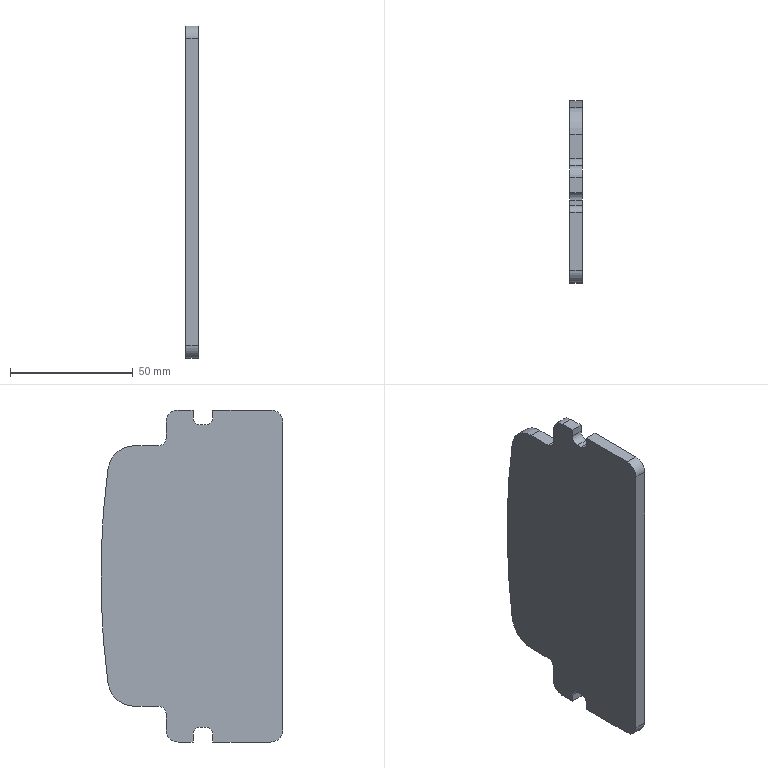Part | SolidWorks | features BaseBody 1 | 1 solid | 30 faces | box 5 x 74 x 135 mm | volume 44638 mm3 | plane 17 | cylinder 13 | commonest cylinder face diameters 6 x6 10 x4 22 x2 660 x1
STEP:
#1=CARTESIAN_POINT('',(616.,51.,53.));
#2=VERTEX_POINT('',#1);
#3=CARTESIAN_POINT('',(616.,48.,56.));
#4=VERTEX_POINT('',#3);
#5=CARTESIAN_POINT('',(616.,51.,56.));
#6=DIRECTION('',(-1.,0.,0.));
#7=DIRECTION('',(0.,0.,-1.));
#8=AXIS2_PLACEMENT_3D('',#5,#6,#7);
#9=CIRCLE('',#8,3.);
#10=EDGE_CURVE('',#2,#4,#9,.T.);
#11=ORIENTED_EDGE('',*,*,#10,.T.);
#12=CARTESIAN_POINT('',(616.,48.,62.5));
#13=VERTEX_POINT('',#12);
#14=CARTESIAN_POINT('',(616.,48.,62.5));
#15=DIRECTION('',(0.,0.,1.));
#16=VECTOR('',#15,1000.);
#17=LINE('',#14,#16);
#18=EDGE_CURVE('',#4,#13,#17,.T.);
#19=ORIENTED_EDGE('',*,*,#18,.T.);
#20=CARTESIAN_POINT('',(616.,43.,67.5));
#21=VERTEX_POINT('',#20);
#22=CARTESIAN_POINT('',(616.,43.,62.5));
#23=DIRECTION('',(1.,0.,0.));
#24=DIRECTION('',(0.,0.,-1.));
#25=AXIS2_PLACEMENT_3D('',#22,#23,#24);
#26=CIRCLE('',#25,5.);
#27=EDGE_CURVE('',#13,#21,#26,.T.);
#28=ORIENTED_EDGE('',*,*,#27,.T.);
#29=CARTESIAN_POINT('',(616.,37.,67.5));
#30=VERTEX_POINT('',#29);
#31=CARTESIAN_POINT('',(616.,43.,67.5));
#32=DIRECTION('',(0.,-1.,0.));
#33=VECTOR('',#32,1000.);
#34=LINE('',#31,#33);
#35=EDGE_CURVE('',#21,#30,#34,.T.);
#36=ORIENTED_EDGE('',*,*,#35,.T.);
#37=CARTESIAN_POINT('',(616.,37.,64.5));
#38=VERTEX_POINT('',#37);
#39=CARTESIAN_POINT('',(616.,37.,62.5));
#40=DIRECTION('',(0.,0.,-1.));
#41=VECTOR('',#40,1000.);
#42=LINE('',#39,#41);
#43=EDGE_CURVE('',#30,#38,#42,.T.);
#44=ORIENTED_EDGE('',*,*,#43,.T.);
#45=CARTESIAN_POINT('',(616.,34.,61.5));
#46=VERTEX_POINT('',#45);
#47=CARTESIAN_POINT('',(616.,34.,64.5));
#48=DIRECTION('',(-1.,0.,0.));
#49=DIRECTION('',(0.,0.,-1.));
#50=AXIS2_PLACEMENT_3D('',#47,#48,#49);
#51=CIRCLE('',#50,3.);
#52=EDGE_CURVE('',#38,#46,#51,.T.);
#53=ORIENTED_EDGE('',*,*,#52,.T.);
#54=CARTESIAN_POINT('',(616.,32.,61.5));
#55=VERTEX_POINT('',#54);
#56=CARTESIAN_POINT('',(616.,43.,61.5));
#57=DIRECTION('',(0.,-1.,0.));
#58=VECTOR('',#57,1000.);
#59=LINE('',#56,#58);
#60=EDGE_CURVE('',#46,#55,#59,.T.);
#61=ORIENTED_EDGE('',*,*,#60,.T.);
#62=CARTESIAN_POINT('',(616.,29.,64.5));
#63=VERTEX_POINT('',#62);
#64=CARTESIAN_POINT('',(616.,32.,64.5));
#65=DIRECTION('',(-1.,0.,0.));
#66=DIRECTION('',(0.,0.,-1.));
#67=AXIS2_PLACEMENT_3D('',#64,#65,#66);
#68=CIRCLE('',#67,3.);
#69=EDGE_CURVE('',#55,#63,#68,.T.);
#70=ORIENTED_EDGE('',*,*,#69,.T.);
#71=CARTESIAN_POINT('',(616.,29.,67.5));
#72=VERTEX_POINT('',#71);
#73=CARTESIAN_POINT('',(616.,29.,62.5));
#74=DIRECTION('',(0.,0.,1.));
#75=VECTOR('',#74,1000.);
#76=LINE('',#73,#75);
#77=EDGE_CURVE('',#63,#72,#76,.T.);
#78=ORIENTED_EDGE('',*,*,#77,.T.);
#79=CARTESIAN_POINT('',(616.,5.5,67.5));
#80=VERTEX_POINT('',#79);
#81=CARTESIAN_POINT('',(616.,43.,67.5));
#82=DIRECTION('',(0.,-1.,0.));
#83=VECTOR('',#82,1000.);
#84=LINE('',#81,#83);
#85=EDGE_CURVE('',#72,#80,#84,.T.);
#86=ORIENTED_EDGE('',*,*,#85,.T.);
#87=CARTESIAN_POINT('',(616.,0.5,62.5));
#88=VERTEX_POINT('',#87);
#89=CARTESIAN_POINT('',(616.,5.5,62.5));
#90=DIRECTION('',(1.,0.,0.));
#91=DIRECTION('',(0.,0.,-1.));
#92=AXIS2_PLACEMENT_3D('',#89,#90,#91);
#93=CIRCLE('',#92,5.);
#94=EDGE_CURVE('',#80,#88,#93,.T.);
#95=ORIENTED_EDGE('',*,*,#94,.T.);
#96=CARTESIAN_POINT('',(616.,0.5,-62.5));
#97=VERTEX_POINT('',#96);
#98=CARTESIAN_POINT('',(616.,0.5,62.5));
#99=DIRECTION('',(0.,0.,-1.));
#100=VECTOR('',#99,1000.);
#101=LINE('',#98,#100);
#102=EDGE_CURVE('',#88,#97,#101,.T.);
#103=ORIENTED_EDGE('',*,*,#102,.T.);
#104=CARTESIAN_POINT('',(616.,5.5,-67.5));
#105=VERTEX_POINT('',#104);
#106=CARTESIAN_POINT('',(616.,5.5,-62.5));
#107=DIRECTION('',(1.,0.,0.));
#108=DIRECTION('',(0.,0.,-1.));
#109=AXIS2_PLACEMENT_3D('',#106,#107,#108);
#110=CIRCLE('',#109,5.);
#111=EDGE_CURVE('',#97,#105,#110,.T.);
#112=ORIENTED_EDGE('',*,*,#111,.T.);
#113=CARTESIAN_POINT('',(616.,29.,-67.5));
#114=VERTEX_POINT('',#113);
#115=CARTESIAN_POINT('',(616.,43.,-67.5));
#116=DIRECTION('',(0.,1.,0.));
#117=VECTOR('',#116,1000.);
#118=LINE('',#115,#117);
#119=EDGE_CURVE('',#105,#114,#118,.T.);
#120=ORIENTED_EDGE('',*,*,#119,.T.);
#121=CARTESIAN_POINT('',(616.,29.,-64.5));
#122=VERTEX_POINT('',#121);
#123=CARTESIAN_POINT('',(616.,29.,62.5));
#124=DIRECTION('',(0.,0.,1.));
#125=VECTOR('',#124,1000.);
#126=LINE('',#123,#125);
#127=EDGE_CURVE('',#114,#122,#126,.T.);
#128=ORIENTED_EDGE('',*,*,#127,.T.);
#129=CARTESIAN_POINT('',(616.,32.,-61.5));
#130=VERTEX_POINT('',#129);
#131=CARTESIAN_POINT('',(616.,32.,-64.5));
#132=DIRECTION('',(-1.,0.,0.));
#133=DIRECTION('',(0.,0.,-1.));
#134=AXIS2_PLACEMENT_3D('',#131,#132,#133);
#135=CIRCLE('',#134,3.);
#136=EDGE_CURVE('',#122,#130,#135,.T.);
#137=ORIENTED_EDGE('',*,*,#136,.T.);
#138=CARTESIAN_POINT('',(616.,34.,-61.5));
#139=VERTEX_POINT('',#138);
#140=CARTESIAN_POINT('',(616.,43.,-61.5));
#141=DIRECTION('',(0.,1.,0.));
#142=VECTOR('',#141,1000.);
#143=LINE('',#140,#142);
#144=EDGE_CURVE('',#130,#139,#143,.T.);
#145=ORIENTED_EDGE('',*,*,#144,.T.);
#146=CARTESIAN_POINT('',(616.,37.,-64.5));
#147=VERTEX_POINT('',#146);
#148=CARTESIAN_POINT('',(616.,34.,-64.5));
#149=DIRECTION('',(-1.,0.,0.));
#150=DIRECTION('',(0.,0.,-1.));
#151=AXIS2_PLACEMENT_3D('',#148,#149,#150);
#152=CIRCLE('',#151,3.);
#153=EDGE_CURVE('',#139,#147,#152,.T.);
#154=ORIENTED_EDGE('',*,*,#153,.T.);
#155=CARTESIAN_POINT('',(616.,37.,-67.5));
#156=VERTEX_POINT('',#155);
#157=CARTESIAN_POINT('',(616.,37.,62.5));
#158=DIRECTION('',(0.,0.,-1.));
#159=VECTOR('',#158,1000.);
#160=LINE('',#157,#159);
#161=EDGE_CURVE('',#147,#156,#160,.T.);
#162=ORIENTED_EDGE('',*,*,#161,.T.);
#163=CARTESIAN_POINT('',(616.,43.,-67.5));
#164=VERTEX_POINT('',#163);
#165=CARTESIAN_POINT('',(616.,43.,-67.5));
#166=DIRECTION('',(0.,1.,0.));
#167=VECTOR('',#166,1000.);
#168=LINE('',#165,#167);
#169=EDGE_CURVE('',#156,#164,#168,.T.);
#170=ORIENTED_EDGE('',*,*,#169,.T.);
#171=CARTESIAN_POINT('',(616.,48.,-62.5));
#172=VERTEX_POINT('',#171);
#173=CARTESIAN_POINT('',(616.,43.,-62.5));
#174=DIRECTION('',(1.,0.,0.));
#175=DIRECTION('',(0.,0.,-1.));
#176=AXIS2_PLACEMENT_3D('',#173,#174,#175);
#177=CIRCLE('',#176,5.);
#178=EDGE_CURVE('',#164,#172,#177,.T.);
#179=ORIENTED_EDGE('',*,*,#178,.T.);
#180=CARTESIAN_POINT('',(616.,48.,-56.));
#181=VERTEX_POINT('',#180);
#182=CARTESIAN_POINT('',(616.,48.,62.5));
#183=DIRECTION('',(0.,0.,1.));
#184=VECTOR('',#183,1000.);
#185=LINE('',#182,#184);
#186=EDGE_CURVE('',#172,#181,#185,.T.);
#187=ORIENTED_EDGE('',*,*,#186,.T.);
#188=CARTESIAN_POINT('',(616.,51.,-53.));
#189=VERTEX_POINT('',#188);
#190=CARTESIAN_POINT('',(616.,51.,-56.));
#191=DIRECTION('',(-1.,0.,0.));
#192=DIRECTION('',(0.,0.,-1.));
#193=AXIS2_PLACEMENT_3D('',#190,#191,#192);
#194=CIRCLE('',#193,3.);
#195=EDGE_CURVE('',#181,#189,#194,.T.);
#196=ORIENTED_EDGE('',*,*,#195,.T.);
#197=CARTESIAN_POINT('',(616.,60.723,-53.));
#198=VERTEX_POINT('',#197);
#199=CARTESIAN_POINT('',(616.,43.,-53.));
#200=DIRECTION('',(0.,1.,0.));
#201=VECTOR('',#200,1000.);
#202=LINE('',#199,#201);
#203=EDGE_CURVE('',#189,#198,#202,.T.);
#204=ORIENTED_EDGE('',*,*,#203,.T.);
#205=CARTESIAN_POINT('',(616.,71.627,-43.448));
#206=VERTEX_POINT('',#205);
#207=CARTESIAN_POINT('',(616.,60.723,-42.));
#208=DIRECTION('',(1.,0.,0.));
#209=DIRECTION('',(0.,0.,-1.));
#210=AXIS2_PLACEMENT_3D('',#207,#208,#209);
#211=CIRCLE('',#210,11.);
#212=EDGE_CURVE('',#198,#206,#211,.T.);
#213=ORIENTED_EDGE('',*,*,#212,.T.);
#214=CARTESIAN_POINT('',(616.,71.627,43.448));
#215=VERTEX_POINT('',#214);
#216=CARTESIAN_POINT('',(616.,-255.5,0.));
#217=DIRECTION('',(1.,0.,0.));
#218=DIRECTION('',(0.,0.,-1.));
#219=AXIS2_PLACEMENT_3D('',#216,#217,#218);
#220=CIRCLE('',#219,330.);
#221=EDGE_CURVE('',#206,#215,#220,.T.);
#222=ORIENTED_EDGE('',*,*,#221,.T.);
#223=CARTESIAN_POINT('',(616.,60.723,53.));
#224=VERTEX_POINT('',#223);
#225=CARTESIAN_POINT('',(616.,60.723,42.));
#226=DIRECTION('',(1.,0.,0.));
#227=DIRECTION('',(0.,0.,-1.));
#228=AXIS2_PLACEMENT_3D('',#225,#226,#227);
#229=CIRCLE('',#228,11.);
#230=EDGE_CURVE('',#215,#224,#229,.T.);
#231=ORIENTED_EDGE('',*,*,#230,.T.);
#232=CARTESIAN_POINT('',(616.,43.,53.));
#233=DIRECTION('',(0.,-1.,0.));
#234=VECTOR('',#233,1000.);
#235=LINE('',#232,#234);
#236=EDGE_CURVE('',#224,#2,#235,.T.);
#237=ORIENTED_EDGE('',*,*,#236,.T.);
#238=EDGE_LOOP('',(#11,#19,#28,#36,#44,#53,#61,#70,#78,#86,#95,#103,#112,#120,#128,#137,#145,#154,#162,#170,#179,#187,#196,#204,#213,#222,#231,#237));
#239=FACE_OUTER_BOUND('',#238,.T.);
#240=CARTESIAN_POINT('',(616.,43.,62.5));
#241=DIRECTION('',(1.,0.,0.));
#242=DIRECTION('',(0.,0.,-1.));
#243=AXIS2_PLACEMENT_3D('',#240,#241,#242);
#244=PLANE('',#243);
#245=ADVANCED_FACE('',(#239),#244,.T.);
#246=CARTESIAN_POINT('',(611.,48.,62.5));
#247=VERTEX_POINT('',#246);
#248=CARTESIAN_POINT('',(616.,48.,62.5));
#249=DIRECTION('',(-1.,0.,0.));
#250=VECTOR('',#249,1000.);
#251=LINE('',#248,#250);
#252=EDGE_CURVE('',#13,#247,#251,.T.);
#253=ORIENTED_EDGE('',*,*,#252,.F.);
#254=ORIENTED_EDGE('',*,*,#18,.F.);
#255=CARTESIAN_POINT('',(611.,48.,56.));
#256=VERTEX_POINT('',#255);
#257=CARTESIAN_POINT('',(616.,48.,56.));
#258=DIRECTION('',(1.,0.,0.));
#259=VECTOR('',#258,1000.);
#260=LINE('',#257,#259);
#261=EDGE_CURVE('',#256,#4,#260,.T.);
#262=ORIENTED_EDGE('',*,*,#261,.F.);
#263=CARTESIAN_POINT('',(611.,48.,56.));
#264=DIRECTION('',(0.,0.,-1.));
#265=VECTOR('',#264,1000.);
#266=LINE('',#263,#265);
#267=EDGE_CURVE('',#247,#256,#266,.T.);
#268=ORIENTED_EDGE('',*,*,#267,.F.);
#269=EDGE_LOOP('',(#253,#254,#262,#268));
#270=FACE_OUTER_BOUND('',#269,.T.);
#271=CARTESIAN_POINT('',(616.,48.,56.));
#272=DIRECTION('',(0.,-1.,0.));
#273=DIRECTION('',(0.,0.,-1.));
#274=AXIS2_PLACEMENT_3D('',#271,#272,#273);
#275=PLANE('',#274);
#276=ADVANCED_FACE('',(#270),#275,.F.);
#277=ORIENTED_EDGE('',*,*,#261,.T.);
#278=ORIENTED_EDGE('',*,*,#10,.F.);
#279=CARTESIAN_POINT('',(611.,51.,53.));
#280=VERTEX_POINT('',#279);
#281=CARTESIAN_POINT('',(616.,51.,53.));
#282=DIRECTION('',(1.,0.,0.));
#283=VECTOR('',#282,1000.);
#284=LINE('',#281,#283);
#285=EDGE_CURVE('',#280,#2,#284,.T.);
#286=ORIENTED_EDGE('',*,*,#285,.F.);
#287=CARTESIAN_POINT('',(611.,51.,56.));
#288=DIRECTION('',(1.,0.,0.));
#289=DIRECTION('',(0.,0.,-1.));
#290=AXIS2_PLACEMENT_3D('',#287,#288,#289);
#291=CIRCLE('',#290,3.);
#292=EDGE_CURVE('',#256,#280,#291,.T.);
#293=ORIENTED_EDGE('',*,*,#292,.F.);
#294=EDGE_LOOP('',(#277,#278,#286,#293));
#295=FACE_OUTER_BOUND('',#294,.T.);
#296=CARTESIAN_POINT('',(616.,51.,56.));
#297=DIRECTION('',(1.,0.,0.));
#298=DIRECTION('',(0.,0.,-1.));
#299=AXIS2_PLACEMENT_3D('',#296,#297,#298);
#300=CYLINDRICAL_SURFACE('',#299,3.);
#301=ADVANCED_FACE('',(#295),#300,.F.);
#302=ORIENTED_EDGE('',*,*,#285,.T.);
#303=ORIENTED_EDGE('',*,*,#236,.F.);
#304=CARTESIAN_POINT('',(611.,60.723,53.));
#305=VERTEX_POINT('',#304);
#306=CARTESIAN_POINT('',(616.,60.723,53.));
#307=DIRECTION('',(1.,0.,0.));
#308=VECTOR('',#307,1000.);
#309=LINE('',#306,#308);
#310=EDGE_CURVE('',#305,#224,#309,.T.);
#311=ORIENTED_EDGE('',*,*,#310,.F.);
#312=CARTESIAN_POINT('',(611.,60.723,53.));
#313=DIRECTION('',(0.,1.,0.));
#314=VECTOR('',#313,1000.);
#315=LINE('',#312,#314);
#316=EDGE_CURVE('',#280,#305,#315,.T.);
#317=ORIENTED_EDGE('',*,*,#316,.F.);
#318=EDGE_LOOP('',(#302,#303,#311,#317));
#319=FACE_OUTER_BOUND('',#318,.T.);
#320=CARTESIAN_POINT('',(616.,60.723,53.));
#321=DIRECTION('',(0.,0.,-1.));
#322=DIRECTION('',(-1.,0.,0.));
#323=AXIS2_PLACEMENT_3D('',#320,#321,#322);
#324=PLANE('',#323);
#325=ADVANCED_FACE('',(#319),#324,.F.);
#326=ORIENTED_EDGE('',*,*,#230,.F.);
#327=CARTESIAN_POINT('',(611.,71.627,43.448));
#328=VERTEX_POINT('',#327);
#329=CARTESIAN_POINT('',(616.,71.627,43.448));
#330=DIRECTION('',(-1.,0.,0.));
#331=VECTOR('',#330,1000.);
#332=LINE('',#329,#331);
#333=EDGE_CURVE('',#215,#328,#332,.T.);
#334=ORIENTED_EDGE('',*,*,#333,.T.);
#335=CARTESIAN_POINT('',(611.,60.723,42.));
#336=DIRECTION('',(1.,0.,0.));
#337=DIRECTION('',(0.,0.,-1.));
#338=AXIS2_PLACEMENT_3D('',#335,#336,#337);
#339=CIRCLE('',#338,11.);
#340=EDGE_CURVE('',#328,#305,#339,.T.);
#341=ORIENTED_EDGE('',*,*,#340,.T.);
#342=ORIENTED_EDGE('',*,*,#310,.T.);
#343=EDGE_LOOP('',(#326,#334,#341,#342));
#344=FACE_OUTER_BOUND('',#343,.T.);
#345=CARTESIAN_POINT('',(616.,60.723,42.));
#346=DIRECTION('',(1.,0.,0.));
#347=DIRECTION('',(0.,0.,-1.));
#348=AXIS2_PLACEMENT_3D('',#345,#346,#347);
#349=CYLINDRICAL_SURFACE('',#348,11.);
#350=ADVANCED_FACE('',(#344),#349,.T.);
#351=ORIENTED_EDGE('',*,*,#221,.F.);
#352=CARTESIAN_POINT('',(611.,71.627,-43.448));
#353=VERTEX_POINT('',#352);
#354=CARTESIAN_POINT('',(616.,71.627,-43.448));
#355=DIRECTION('',(-1.,0.,0.));
#356=VECTOR('',#355,1000.);
#357=LINE('',#354,#356);
#358=EDGE_CURVE('',#206,#353,#357,.T.);
#359=ORIENTED_EDGE('',*,*,#358,.T.);
#360=CARTESIAN_POINT('',(611.,-255.5,0.));
#361=DIRECTION('',(1.,0.,0.));
#362=DIRECTION('',(0.,0.,-1.));
#363=AXIS2_PLACEMENT_3D('',#360,#361,#362);
#364=CIRCLE('',#363,330.);
#365=EDGE_CURVE('',#353,#328,#364,.T.);
#366=ORIENTED_EDGE('',*,*,#365,.T.);
#367=ORIENTED_EDGE('',*,*,#333,.F.);
#368=EDGE_LOOP('',(#351,#359,#366,#367));
#369=FACE_OUTER_BOUND('',#368,.T.);
#370=CARTESIAN_POINT('',(616.,-255.5,0.));
#371=DIRECTION('',(1.,0.,0.));
#372=DIRECTION('',(0.,0.,-1.));
#373=AXIS2_PLACEMENT_3D('',#370,#371,#372);
#374=CYLINDRICAL_SURFACE('',#373,330.);
#375=ADVANCED_FACE('',(#369),#374,.T.);
#376=ORIENTED_EDGE('',*,*,#212,.F.);
#377=CARTESIAN_POINT('',(611.,60.723,-53.));
#378=VERTEX_POINT('',#377);
#379=CARTESIAN_POINT('',(616.,60.723,-53.));
#380=DIRECTION('',(-1.,0.,0.));
#381=VECTOR('',#380,1000.);
#382=LINE('',#379,#381);
#383=EDGE_CURVE('',#198,#378,#382,.T.);
#384=ORIENTED_EDGE('',*,*,#383,.T.);
#385=CARTESIAN_POINT('',(611.,60.723,-42.));
#386=DIRECTION('',(1.,0.,0.));
#387=DIRECTION('',(0.,0.,-1.));
#388=AXIS2_PLACEMENT_3D('',#385,#386,#387);
#389=CIRCLE('',#388,11.);
#390=EDGE_CURVE('',#378,#353,#389,.T.);
#391=ORIENTED_EDGE('',*,*,#390,.T.);
#392=ORIENTED_EDGE('',*,*,#358,.F.);
#393=EDGE_LOOP('',(#376,#384,#391,#392));
#394=FACE_OUTER_BOUND('',#393,.T.);
#395=CARTESIAN_POINT('',(616.,60.723,-42.));
#396=DIRECTION('',(1.,0.,0.));
#397=DIRECTION('',(0.,0.,-1.));
#398=AXIS2_PLACEMENT_3D('',#395,#396,#397);
#399=CYLINDRICAL_SURFACE('',#398,11.);
#400=ADVANCED_FACE('',(#394),#399,.T.);
#401=ORIENTED_EDGE('',*,*,#383,.F.);
#402=ORIENTED_EDGE('',*,*,#203,.F.);
#403=CARTESIAN_POINT('',(611.,51.,-53.));
#404=VERTEX_POINT('',#403);
#405=CARTESIAN_POINT('',(616.,51.,-53.));
#406=DIRECTION('',(1.,0.,0.));
#407=VECTOR('',#406,1000.);
#408=LINE('',#405,#407);
#409=EDGE_CURVE('',#404,#189,#408,.T.);
#410=ORIENTED_EDGE('',*,*,#409,.F.);
#411=CARTESIAN_POINT('',(611.,51.,-53.));
#412=DIRECTION('',(0.,-1.,0.));
#413=VECTOR('',#412,1000.);
#414=LINE('',#411,#413);
#415=EDGE_CURVE('',#378,#404,#414,.T.);
#416=ORIENTED_EDGE('',*,*,#415,.F.);
#417=EDGE_LOOP('',(#401,#402,#410,#416));
#418=FACE_OUTER_BOUND('',#417,.T.);
#419=CARTESIAN_POINT('',(616.,51.,-53.));
#420=DIRECTION('',(0.,0.,1.));
#421=DIRECTION('',(1.,0.,0.));
#422=AXIS2_PLACEMENT_3D('',#419,#420,#421);
#423=PLANE('',#422);
#424=ADVANCED_FACE('',(#418),#423,.F.);
#425=ORIENTED_EDGE('',*,*,#409,.T.);
#426=ORIENTED_EDGE('',*,*,#195,.F.);
#427=CARTESIAN_POINT('',(611.,48.,-56.));
#428=VERTEX_POINT('',#427);
#429=CARTESIAN_POINT('',(616.,48.,-56.));
#430=DIRECTION('',(1.,0.,0.));
#431=VECTOR('',#430,1000.);
#432=LINE('',#429,#431);
#433=EDGE_CURVE('',#428,#181,#432,.T.);
#434=ORIENTED_EDGE('',*,*,#433,.F.);
#435=CARTESIAN_POINT('',(611.,51.,-56.));
#436=DIRECTION('',(1.,0.,0.));
#437=DIRECTION('',(0.,0.,-1.));
#438=AXIS2_PLACEMENT_3D('',#435,#436,#437);
#439=CIRCLE('',#438,3.);
#440=EDGE_CURVE('',#404,#428,#439,.T.);
#441=ORIENTED_EDGE('',*,*,#440,.F.);
#442=EDGE_LOOP('',(#425,#426,#434,#441));
#443=FACE_OUTER_BOUND('',#442,.T.);
#444=CARTESIAN_POINT('',(616.,51.,-56.));
#445=DIRECTION('',(1.,0.,0.));
#446=DIRECTION('',(0.,0.,-1.));
#447=AXIS2_PLACEMENT_3D('',#444,#445,#446);
#448=CYLINDRICAL_SURFACE('',#447,3.);
#449=ADVANCED_FACE('',(#443),#448,.F.);
#450=ORIENTED_EDGE('',*,*,#433,.T.);
#451=ORIENTED_EDGE('',*,*,#186,.F.);
#452=CARTESIAN_POINT('',(611.,48.,-62.5));
#453=VERTEX_POINT('',#452);
#454=CARTESIAN_POINT('',(616.,48.,-62.5));
#455=DIRECTION('',(1.,0.,0.));
#456=VECTOR('',#455,1000.);
#457=LINE('',#454,#456);
#458=EDGE_CURVE('',#453,#172,#457,.T.);
#459=ORIENTED_EDGE('',*,*,#458,.F.);
#460=CARTESIAN_POINT('',(611.,48.,-62.5));
#461=DIRECTION('',(0.,0.,-1.));
#462=VECTOR('',#461,1000.);
#463=LINE('',#460,#462);
#464=EDGE_CURVE('',#428,#453,#463,.T.);
#465=ORIENTED_EDGE('',*,*,#464,.F.);
#466=EDGE_LOOP('',(#450,#451,#459,#465));
#467=FACE_OUTER_BOUND('',#466,.T.);
#468=CARTESIAN_POINT('',(616.,48.,-62.5));
#469=DIRECTION('',(0.,-1.,0.));
#470=DIRECTION('',(0.,0.,-1.));
#471=AXIS2_PLACEMENT_3D('',#468,#469,#470);
#472=PLANE('',#471);
#473=ADVANCED_FACE('',(#467),#472,.F.);
#474=ORIENTED_EDGE('',*,*,#178,.F.);
#475=CARTESIAN_POINT('',(611.,43.,-67.5));
#476=VERTEX_POINT('',#475);
#477=CARTESIAN_POINT('',(616.,43.,-67.5));
#478=DIRECTION('',(-1.,0.,0.));
#479=VECTOR('',#478,1000.);
#480=LINE('',#477,#479);
#481=EDGE_CURVE('',#164,#476,#480,.T.);
#482=ORIENTED_EDGE('',*,*,#481,.T.);
#483=CARTESIAN_POINT('',(611.,43.,-62.5));
#484=DIRECTION('',(1.,0.,0.));
#485=DIRECTION('',(0.,0.,-1.));
#486=AXIS2_PLACEMENT_3D('',#483,#484,#485);
#487=CIRCLE('',#486,5.);
#488=EDGE_CURVE('',#476,#453,#487,.T.);
#489=ORIENTED_EDGE('',*,*,#488,.T.);
#490=ORIENTED_EDGE('',*,*,#458,.T.);
#491=EDGE_LOOP('',(#474,#482,#489,#490));
#492=FACE_OUTER_BOUND('',#491,.T.);
#493=CARTESIAN_POINT('',(616.,43.,-62.5));
#494=DIRECTION('',(1.,0.,0.));
#495=DIRECTION('',(0.,0.,-1.));
#496=AXIS2_PLACEMENT_3D('',#493,#494,#495);
#497=CYLINDRICAL_SURFACE('',#496,5.);
#498=ADVANCED_FACE('',(#492),#497,.T.);
#499=ORIENTED_EDGE('',*,*,#481,.F.);
#500=ORIENTED_EDGE('',*,*,#169,.F.);
#501=CARTESIAN_POINT('',(611.,37.,-67.5));
#502=VERTEX_POINT('',#501);
#503=CARTESIAN_POINT('',(616.,37.,-67.5));
#504=DIRECTION('',(1.,0.,0.));
#505=VECTOR('',#504,1000.);
#506=LINE('',#503,#505);
#507=EDGE_CURVE('',#502,#156,#506,.T.);
#508=ORIENTED_EDGE('',*,*,#507,.F.);
#509=CARTESIAN_POINT('',(611.,37.,-67.5));
#510=DIRECTION('',(0.,-1.,0.));
#511=VECTOR('',#510,1000.);
#512=LINE('',#509,#511);
#513=EDGE_CURVE('',#476,#502,#512,.T.);
#514=ORIENTED_EDGE('',*,*,#513,.F.);
#515=EDGE_LOOP('',(#499,#500,#508,#514));
#516=FACE_OUTER_BOUND('',#515,.T.);
#517=CARTESIAN_POINT('',(616.,37.,-67.5));
#518=DIRECTION('',(0.,0.,1.));
#519=DIRECTION('',(1.,0.,0.));
#520=AXIS2_PLACEMENT_3D('',#517,#518,#519);
#521=PLANE('',#520);
#522=ADVANCED_FACE('',(#516),#521,.F.);
#523=ORIENTED_EDGE('',*,*,#507,.T.);
#524=ORIENTED_EDGE('',*,*,#161,.F.);
#525=CARTESIAN_POINT('',(611.,37.,-64.5));
#526=VERTEX_POINT('',#525);
#527=CARTESIAN_POINT('',(616.,37.,-64.5));
#528=DIRECTION('',(1.,0.,0.));
#529=VECTOR('',#528,1000.);
#530=LINE('',#527,#529);
#531=EDGE_CURVE('',#526,#147,#530,.T.);
#532=ORIENTED_EDGE('',*,*,#531,.F.);
#533=CARTESIAN_POINT('',(611.,37.,-64.5));
#534=DIRECTION('',(0.,0.,1.));
#535=VECTOR('',#534,1000.);
#536=LINE('',#533,#535);
#537=EDGE_CURVE('',#502,#526,#536,.T.);
#538=ORIENTED_EDGE('',*,*,#537,.F.);
#539=EDGE_LOOP('',(#523,#524,#532,#538));
#540=FACE_OUTER_BOUND('',#539,.T.);
#541=CARTESIAN_POINT('',(616.,37.,-64.5));
#542=DIRECTION('',(0.,1.,0.));
#543=DIRECTION('',(0.,0.,1.));
#544=AXIS2_PLACEMENT_3D('',#541,#542,#543);
#545=PLANE('',#544);
#546=ADVANCED_FACE('',(#540),#545,.F.);
#547=ORIENTED_EDGE('',*,*,#531,.T.);
#548=ORIENTED_EDGE('',*,*,#153,.F.);
#549=CARTESIAN_POINT('',(611.,34.,-61.5));
#550=VERTEX_POINT('',#549);
#551=CARTESIAN_POINT('',(616.,34.,-61.5));
#552=DIRECTION('',(1.,0.,0.));
#553=VECTOR('',#552,1000.);
#554=LINE('',#551,#553);
#555=EDGE_CURVE('',#550,#139,#554,.T.);
#556=ORIENTED_EDGE('',*,*,#555,.F.);
#557=CARTESIAN_POINT('',(611.,34.,-64.5));
#558=DIRECTION('',(1.,0.,0.));
#559=DIRECTION('',(0.,0.,-1.));
#560=AXIS2_PLACEMENT_3D('',#557,#558,#559);
#561=CIRCLE('',#560,3.);
#562=EDGE_CURVE('',#526,#550,#561,.T.);
#563=ORIENTED_EDGE('',*,*,#562,.F.);
#564=EDGE_LOOP('',(#547,#548,#556,#563));
#565=FACE_OUTER_BOUND('',#564,.T.);
#566=CARTESIAN_POINT('',(616.,34.,-64.5));
#567=DIRECTION('',(1.,0.,0.));
#568=DIRECTION('',(0.,0.,-1.));
#569=AXIS2_PLACEMENT_3D('',#566,#567,#568);
#570=CYLINDRICAL_SURFACE('',#569,3.);
#571=ADVANCED_FACE('',(#565),#570,.F.);
#572=ORIENTED_EDGE('',*,*,#555,.T.);
#573=ORIENTED_EDGE('',*,*,#144,.F.);
#574=CARTESIAN_POINT('',(611.,32.,-61.5));
#575=VERTEX_POINT('',#574);
#576=CARTESIAN_POINT('',(616.,32.,-61.5));
#577=DIRECTION('',(1.,0.,0.));
#578=VECTOR('',#577,1000.);
#579=LINE('',#576,#578);
#580=EDGE_CURVE('',#575,#130,#579,.T.);
#581=ORIENTED_EDGE('',*,*,#580,.F.);
#582=CARTESIAN_POINT('',(611.,32.,-61.5));
#583=DIRECTION('',(0.,-1.,0.));
#584=VECTOR('',#583,1000.);
#585=LINE('',#582,#584);
#586=EDGE_CURVE('',#550,#575,#585,.T.);
#587=ORIENTED_EDGE('',*,*,#586,.F.);
#588=EDGE_LOOP('',(#572,#573,#581,#587));
#589=FACE_OUTER_BOUND('',#588,.T.);
#590=CARTESIAN_POINT('',(616.,32.,-61.5));
#591=DIRECTION('',(0.,0.,1.));
#592=DIRECTION('',(1.,0.,0.));
#593=AXIS2_PLACEMENT_3D('',#590,#591,#592);
#594=PLANE('',#593);
#595=ADVANCED_FACE('',(#589),#594,.F.);
#596=ORIENTED_EDGE('',*,*,#580,.T.);
#597=ORIENTED_EDGE('',*,*,#136,.F.);
#598=CARTESIAN_POINT('',(611.,29.,-64.5));
#599=VERTEX_POINT('',#598);
#600=CARTESIAN_POINT('',(616.,29.,-64.5));
#601=DIRECTION('',(1.,0.,0.));
#602=VECTOR('',#601,1000.);
#603=LINE('',#600,#602);
#604=EDGE_CURVE('',#599,#122,#603,.T.);
#605=ORIENTED_EDGE('',*,*,#604,.F.);
#606=CARTESIAN_POINT('',(611.,32.,-64.5));
#607=DIRECTION('',(1.,0.,0.));
#608=DIRECTION('',(0.,0.,-1.));
#609=AXIS2_PLACEMENT_3D('',#606,#607,#608);
#610=CIRCLE('',#609,3.);
#611=EDGE_CURVE('',#575,#599,#610,.T.);
#612=ORIENTED_EDGE('',*,*,#611,.F.);
#613=EDGE_LOOP('',(#596,#597,#605,#612));
#614=FACE_OUTER_BOUND('',#613,.T.);
#615=CARTESIAN_POINT('',(616.,32.,-64.5));
#616=DIRECTION('',(1.,0.,0.));
#617=DIRECTION('',(0.,0.,-1.));
#618=AXIS2_PLACEMENT_3D('',#615,#616,#617);
#619=CYLINDRICAL_SURFACE('',#618,3.);
#620=ADVANCED_FACE('',(#614),#619,.F.);
#621=ORIENTED_EDGE('',*,*,#604,.T.);
#622=ORIENTED_EDGE('',*,*,#127,.F.);
#623=CARTESIAN_POINT('',(611.,29.,-67.5));
#624=VERTEX_POINT('',#623);
#625=CARTESIAN_POINT('',(616.,29.,-67.5));
#626=DIRECTION('',(1.,0.,0.));
#627=VECTOR('',#626,1000.);
#628=LINE('',#625,#627);
#629=EDGE_CURVE('',#624,#114,#628,.T.);
#630=ORIENTED_EDGE('',*,*,#629,.F.);
#631=CARTESIAN_POINT('',(611.,29.,-67.5));
#632=DIRECTION('',(0.,0.,-1.));
#633=VECTOR('',#632,1000.);
#634=LINE('',#631,#633);
#635=EDGE_CURVE('',#599,#624,#634,.T.);
#636=ORIENTED_EDGE('',*,*,#635,.F.);
#637=EDGE_LOOP('',(#621,#622,#630,#636));
#638=FACE_OUTER_BOUND('',#637,.T.);
#639=CARTESIAN_POINT('',(616.,29.,-67.5));
#640=DIRECTION('',(0.,-1.,0.));
#641=DIRECTION('',(0.,0.,-1.));
#642=AXIS2_PLACEMENT_3D('',#639,#640,#641);
#643=PLANE('',#642);
#644=ADVANCED_FACE('',(#638),#643,.F.);
#645=ORIENTED_EDGE('',*,*,#629,.T.);
#646=ORIENTED_EDGE('',*,*,#119,.F.);
#647=CARTESIAN_POINT('',(611.,5.5,-67.5));
#648=VERTEX_POINT('',#647);
#649=CARTESIAN_POINT('',(616.,5.5,-67.5));
#650=DIRECTION('',(1.,0.,0.));
#651=VECTOR('',#650,1000.);
#652=LINE('',#649,#651);
#653=EDGE_CURVE('',#648,#105,#652,.T.);
#654=ORIENTED_EDGE('',*,*,#653,.F.);
#655=CARTESIAN_POINT('',(611.,5.5,-67.5));
#656=DIRECTION('',(0.,-1.,0.));
#657=VECTOR('',#656,1000.);
#658=LINE('',#655,#657);
#659=EDGE_CURVE('',#624,#648,#658,.T.);
#660=ORIENTED_EDGE('',*,*,#659,.F.);
#661=EDGE_LOOP('',(#645,#646,#654,#660));
#662=FACE_OUTER_BOUND('',#661,.T.);
#663=CARTESIAN_POINT('',(616.,5.5,-67.5));
#664=DIRECTION('',(0.,0.,1.));
#665=DIRECTION('',(1.,0.,0.));
#666=AXIS2_PLACEMENT_3D('',#663,#664,#665);
#667=PLANE('',#666);
#668=ADVANCED_FACE('',(#662),#667,.F.);
#669=ORIENTED_EDGE('',*,*,#111,.F.);
#670=CARTESIAN_POINT('',(611.,0.5,-62.5));
#671=VERTEX_POINT('',#670);
#672=CARTESIAN_POINT('',(616.,0.5,-62.5));
#673=DIRECTION('',(-1.,0.,0.));
#674=VECTOR('',#673,1000.);
#675=LINE('',#672,#674);
#676=EDGE_CURVE('',#97,#671,#675,.T.);
#677=ORIENTED_EDGE('',*,*,#676,.T.);
#678=CARTESIAN_POINT('',(611.,5.5,-62.5));
#679=DIRECTION('',(1.,0.,0.));
#680=DIRECTION('',(0.,0.,-1.));
#681=AXIS2_PLACEMENT_3D('',#678,#679,#680);
#682=CIRCLE('',#681,5.);
#683=EDGE_CURVE('',#671,#648,#682,.T.);
#684=ORIENTED_EDGE('',*,*,#683,.T.);
#685=ORIENTED_EDGE('',*,*,#653,.T.);
#686=EDGE_LOOP('',(#669,#677,#684,#685));
#687=FACE_OUTER_BOUND('',#686,.T.);
#688=CARTESIAN_POINT('',(616.,5.5,-62.5));
#689=DIRECTION('',(1.,0.,0.));
#690=DIRECTION('',(0.,0.,-1.));
#691=AXIS2_PLACEMENT_3D('',#688,#689,#690);
#692=CYLINDRICAL_SURFACE('',#691,5.);
#693=ADVANCED_FACE('',(#687),#692,.T.);
#694=ORIENTED_EDGE('',*,*,#676,.F.);
#695=ORIENTED_EDGE('',*,*,#102,.F.);
#696=CARTESIAN_POINT('',(611.,0.5,62.5));
#697=VERTEX_POINT('',#696);
#698=CARTESIAN_POINT('',(616.,0.5,62.5));
#699=DIRECTION('',(1.,0.,0.));
#700=VECTOR('',#699,1000.);
#701=LINE('',#698,#700);
#702=EDGE_CURVE('',#697,#88,#701,.T.);
#703=ORIENTED_EDGE('',*,*,#702,.F.);
#704=CARTESIAN_POINT('',(611.,0.5,62.5));
#705=DIRECTION('',(0.,0.,1.));
#706=VECTOR('',#705,1000.);
#707=LINE('',#704,#706);
#708=EDGE_CURVE('',#671,#697,#707,.T.);
#709=ORIENTED_EDGE('',*,*,#708,.F.);
#710=EDGE_LOOP('',(#694,#695,#703,#709));
#711=FACE_OUTER_BOUND('',#710,.T.);
#712=CARTESIAN_POINT('',(616.,0.5,62.5));
#713=DIRECTION('',(0.,1.,0.));
#714=DIRECTION('',(0.,0.,1.));
#715=AXIS2_PLACEMENT_3D('',#712,#713,#714);
#716=PLANE('',#715);
#717=ADVANCED_FACE('',(#711),#716,.F.);
#718=ORIENTED_EDGE('',*,*,#94,.F.);
#719=CARTESIAN_POINT('',(611.,5.5,67.5));
#720=VERTEX_POINT('',#719);
#721=CARTESIAN_POINT('',(616.,5.5,67.5));
#722=DIRECTION('',(-1.,0.,0.));
#723=VECTOR('',#722,1000.);
#724=LINE('',#721,#723);
#725=EDGE_CURVE('',#80,#720,#724,.T.);
#726=ORIENTED_EDGE('',*,*,#725,.T.);
#727=CARTESIAN_POINT('',(611.,5.5,62.5));
#728=DIRECTION('',(1.,0.,0.));
#729=DIRECTION('',(0.,0.,-1.));
#730=AXIS2_PLACEMENT_3D('',#727,#728,#729);
#731=CIRCLE('',#730,5.);
#732=EDGE_CURVE('',#720,#697,#731,.T.);
#733=ORIENTED_EDGE('',*,*,#732,.T.);
#734=ORIENTED_EDGE('',*,*,#702,.T.);
#735=EDGE_LOOP('',(#718,#726,#733,#734));
#736=FACE_OUTER_BOUND('',#735,.T.);
#737=CARTESIAN_POINT('',(616.,5.5,62.5));
#738=DIRECTION('',(1.,0.,0.));
#739=DIRECTION('',(0.,0.,-1.));
#740=AXIS2_PLACEMENT_3D('',#737,#738,#739);
#741=CYLINDRICAL_SURFACE('',#740,5.);
#742=ADVANCED_FACE('',(#736),#741,.T.);
#743=ORIENTED_EDGE('',*,*,#725,.F.);
#744=ORIENTED_EDGE('',*,*,#85,.F.);
#745=CARTESIAN_POINT('',(611.,29.,67.5));
#746=VERTEX_POINT('',#745);
#747=CARTESIAN_POINT('',(616.,29.,67.5));
#748=DIRECTION('',(1.,0.,0.));
#749=VECTOR('',#748,1000.);
#750=LINE('',#747,#749);
#751=EDGE_CURVE('',#746,#72,#750,.T.);
#752=ORIENTED_EDGE('',*,*,#751,.F.);
#753=CARTESIAN_POINT('',(611.,29.,67.5));
#754=DIRECTION('',(0.,1.,0.));
#755=VECTOR('',#754,1000.);
#756=LINE('',#753,#755);
#757=EDGE_CURVE('',#720,#746,#756,.T.);
#758=ORIENTED_EDGE('',*,*,#757,.F.);
#759=EDGE_LOOP('',(#743,#744,#752,#758));
#760=FACE_OUTER_BOUND('',#759,.T.);
#761=CARTESIAN_POINT('',(616.,29.,67.5));
#762=DIRECTION('',(0.,0.,-1.));
#763=DIRECTION('',(-1.,0.,0.));
#764=AXIS2_PLACEMENT_3D('',#761,#762,#763);
#765=PLANE('',#764);
#766=ADVANCED_FACE('',(#760),#765,.F.);
#767=ORIENTED_EDGE('',*,*,#751,.T.);
#768=ORIENTED_EDGE('',*,*,#77,.F.);
#769=CARTESIAN_POINT('',(611.,29.,64.5));
#770=VERTEX_POINT('',#769);
#771=CARTESIAN_POINT('',(616.,29.,64.5));
#772=DIRECTION('',(1.,0.,0.));
#773=VECTOR('',#772,1000.);
#774=LINE('',#771,#773);
#775=EDGE_CURVE('',#770,#63,#774,.T.);
#776=ORIENTED_EDGE('',*,*,#775,.F.);
#777=CARTESIAN_POINT('',(611.,29.,64.5));
#778=DIRECTION('',(0.,0.,-1.));
#779=VECTOR('',#778,1000.);
#780=LINE('',#777,#779);
#781=EDGE_CURVE('',#746,#770,#780,.T.);
#782=ORIENTED_EDGE('',*,*,#781,.F.);
#783=EDGE_LOOP('',(#767,#768,#776,#782));
#784=FACE_OUTER_BOUND('',#783,.T.);
#785=CARTESIAN_POINT('',(616.,29.,64.5));
#786=DIRECTION('',(0.,-1.,0.));
#787=DIRECTION('',(0.,0.,-1.));
#788=AXIS2_PLACEMENT_3D('',#785,#786,#787);
#789=PLANE('',#788);
#790=ADVANCED_FACE('',(#784),#789,.F.);
#791=ORIENTED_EDGE('',*,*,#775,.T.);
#792=ORIENTED_EDGE('',*,*,#69,.F.);
#793=CARTESIAN_POINT('',(611.,32.,61.5));
#794=VERTEX_POINT('',#793);
#795=CARTESIAN_POINT('',(616.,32.,61.5));
#796=DIRECTION('',(1.,0.,0.));
#797=VECTOR('',#796,1000.);
#798=LINE('',#795,#797);
#799=EDGE_CURVE('',#794,#55,#798,.T.);
#800=ORIENTED_EDGE('',*,*,#799,.F.);
#801=CARTESIAN_POINT('',(611.,32.,64.5));
#802=DIRECTION('',(1.,0.,0.));
#803=DIRECTION('',(0.,0.,-1.));
#804=AXIS2_PLACEMENT_3D('',#801,#802,#803);
#805=CIRCLE('',#804,3.);
#806=EDGE_CURVE('',#770,#794,#805,.T.);
#807=ORIENTED_EDGE('',*,*,#806,.F.);
#808=EDGE_LOOP('',(#791,#792,#800,#807));
#809=FACE_OUTER_BOUND('',#808,.T.);
#810=CARTESIAN_POINT('',(616.,32.,64.5));
#811=DIRECTION('',(1.,0.,0.));
#812=DIRECTION('',(0.,0.,-1.));
#813=AXIS2_PLACEMENT_3D('',#810,#811,#812);
#814=CYLINDRICAL_SURFACE('',#813,3.);
#815=ADVANCED_FACE('',(#809),#814,.F.);
#816=ORIENTED_EDGE('',*,*,#799,.T.);
#817=ORIENTED_EDGE('',*,*,#60,.F.);
#818=CARTESIAN_POINT('',(611.,34.,61.5));
#819=VERTEX_POINT('',#818);
#820=CARTESIAN_POINT('',(616.,34.,61.5));
#821=DIRECTION('',(1.,0.,0.));
#822=VECTOR('',#821,1000.);
#823=LINE('',#820,#822);
#824=EDGE_CURVE('',#819,#46,#823,.T.);
#825=ORIENTED_EDGE('',*,*,#824,.F.);
#826=CARTESIAN_POINT('',(611.,34.,61.5));
#827=DIRECTION('',(0.,1.,0.));
#828=VECTOR('',#827,1000.);
#829=LINE('',#826,#828);
#830=EDGE_CURVE('',#794,#819,#829,.T.);
#831=ORIENTED_EDGE('',*,*,#830,.F.);
#832=EDGE_LOOP('',(#816,#817,#825,#831));
#833=FACE_OUTER_BOUND('',#832,.T.);
#834=CARTESIAN_POINT('',(616.,34.,61.5));
#835=DIRECTION('',(0.,0.,-1.));
#836=DIRECTION('',(-1.,0.,0.));
#837=AXIS2_PLACEMENT_3D('',#834,#835,#836);
#838=PLANE('',#837);
#839=ADVANCED_FACE('',(#833),#838,.F.);
#840=ORIENTED_EDGE('',*,*,#824,.T.);
#841=ORIENTED_EDGE('',*,*,#52,.F.);
#842=CARTESIAN_POINT('',(611.,37.,64.5));
#843=VERTEX_POINT('',#842);
#844=CARTESIAN_POINT('',(616.,37.,64.5));
#845=DIRECTION('',(1.,0.,0.));
#846=VECTOR('',#845,1000.);
#847=LINE('',#844,#846);
#848=EDGE_CURVE('',#843,#38,#847,.T.);
#849=ORIENTED_EDGE('',*,*,#848,.F.);
#850=CARTESIAN_POINT('',(611.,34.,64.5));
#851=DIRECTION('',(1.,0.,0.));
#852=DIRECTION('',(0.,0.,-1.));
#853=AXIS2_PLACEMENT_3D('',#850,#851,#852);
#854=CIRCLE('',#853,3.);
#855=EDGE_CURVE('',#819,#843,#854,.T.);
#856=ORIENTED_EDGE('',*,*,#855,.F.);
#857=EDGE_LOOP('',(#840,#841,#849,#856));
#858=FACE_OUTER_BOUND('',#857,.T.);
#859=CARTESIAN_POINT('',(616.,34.,64.5));
#860=DIRECTION('',(1.,0.,0.));
#861=DIRECTION('',(0.,0.,-1.));
#862=AXIS2_PLACEMENT_3D('',#859,#860,#861);
#863=CYLINDRICAL_SURFACE('',#862,3.);
#864=ADVANCED_FACE('',(#858),#863,.F.);
#865=ORIENTED_EDGE('',*,*,#848,.T.);
#866=ORIENTED_EDGE('',*,*,#43,.F.);
#867=CARTESIAN_POINT('',(611.,37.,67.5));
#868=VERTEX_POINT('',#867);
#869=CARTESIAN_POINT('',(616.,37.,67.5));
#870=DIRECTION('',(1.,0.,0.));
#871=VECTOR('',#870,1000.);
#872=LINE('',#869,#871);
#873=EDGE_CURVE('',#868,#30,#872,.T.);
#874=ORIENTED_EDGE('',*,*,#873,.F.);
#875=CARTESIAN_POINT('',(611.,37.,67.5));
#876=DIRECTION('',(0.,0.,1.));
#877=VECTOR('',#876,1000.);
#878=LINE('',#875,#877);
#879=EDGE_CURVE('',#843,#868,#878,.T.);
#880=ORIENTED_EDGE('',*,*,#879,.F.);
#881=EDGE_LOOP('',(#865,#866,#874,#880));
#882=FACE_OUTER_BOUND('',#881,.T.);
#883=CARTESIAN_POINT('',(616.,37.,67.5));
#884=DIRECTION('',(0.,1.,0.));
#885=DIRECTION('',(0.,0.,1.));
#886=AXIS2_PLACEMENT_3D('',#883,#884,#885);
#887=PLANE('',#886);
#888=ADVANCED_FACE('',(#882),#887,.F.);
#889=ORIENTED_EDGE('',*,*,#873,.T.);
#890=ORIENTED_EDGE('',*,*,#35,.F.);
#891=CARTESIAN_POINT('',(611.,43.,67.5));
#892=VERTEX_POINT('',#891);
#893=CARTESIAN_POINT('',(616.,43.,67.5));
#894=DIRECTION('',(1.,0.,0.));
#895=VECTOR('',#894,1000.);
#896=LINE('',#893,#895);
#897=EDGE_CURVE('',#892,#21,#896,.T.);
#898=ORIENTED_EDGE('',*,*,#897,.F.);
#899=CARTESIAN_POINT('',(611.,43.,67.5));
#900=DIRECTION('',(0.,1.,0.));
#901=VECTOR('',#900,1000.);
#902=LINE('',#899,#901);
#903=EDGE_CURVE('',#868,#892,#902,.T.);
#904=ORIENTED_EDGE('',*,*,#903,.F.);
#905=EDGE_LOOP('',(#889,#890,#898,#904));
#906=FACE_OUTER_BOUND('',#905,.T.);
#907=CARTESIAN_POINT('',(616.,43.,67.5));
#908=DIRECTION('',(0.,0.,-1.));
#909=DIRECTION('',(-1.,0.,0.));
#910=AXIS2_PLACEMENT_3D('',#907,#908,#909);
#911=PLANE('',#910);
#912=ADVANCED_FACE('',(#906),#911,.F.);
#913=ORIENTED_EDGE('',*,*,#27,.F.);
#914=ORIENTED_EDGE('',*,*,#252,.T.);
#915=CARTESIAN_POINT('',(611.,43.,62.5));
#916=DIRECTION('',(1.,0.,0.));
#917=DIRECTION('',(0.,0.,-1.));
#918=AXIS2_PLACEMENT_3D('',#915,#916,#917);
#919=CIRCLE('',#918,5.);
#920=EDGE_CURVE('',#247,#892,#919,.T.);
#921=ORIENTED_EDGE('',*,*,#920,.T.);
#922=ORIENTED_EDGE('',*,*,#897,.T.);
#923=EDGE_LOOP('',(#913,#914,#921,#922));
#924=FACE_OUTER_BOUND('',#923,.T.);
#925=CARTESIAN_POINT('',(616.,43.,62.5));
#926=DIRECTION('',(1.,0.,0.));
#927=DIRECTION('',(0.,0.,-1.));
#928=AXIS2_PLACEMENT_3D('',#925,#926,#927);
#929=CYLINDRICAL_SURFACE('',#928,5.);
#930=ADVANCED_FACE('',(#924),#929,.T.);
#931=ORIENTED_EDGE('',*,*,#267,.T.);
#932=ORIENTED_EDGE('',*,*,#292,.T.);
#933=ORIENTED_EDGE('',*,*,#316,.T.);
#934=ORIENTED_EDGE('',*,*,#340,.F.);
#935=ORIENTED_EDGE('',*,*,#365,.F.);
#936=ORIENTED_EDGE('',*,*,#390,.F.);
#937=ORIENTED_EDGE('',*,*,#415,.T.);
#938=ORIENTED_EDGE('',*,*,#440,.T.);
#939=ORIENTED_EDGE('',*,*,#464,.T.);
#940=ORIENTED_EDGE('',*,*,#488,.F.);
#941=ORIENTED_EDGE('',*,*,#513,.T.);
#942=ORIENTED_EDGE('',*,*,#537,.T.);
#943=ORIENTED_EDGE('',*,*,#562,.T.);
#944=ORIENTED_EDGE('',*,*,#586,.T.);
#945=ORIENTED_EDGE('',*,*,#611,.T.);
#946=ORIENTED_EDGE('',*,*,#635,.T.);
#947=ORIENTED_EDGE('',*,*,#659,.T.);
#948=ORIENTED_EDGE('',*,*,#683,.F.);
#949=ORIENTED_EDGE('',*,*,#708,.T.);
#950=ORIENTED_EDGE('',*,*,#732,.F.);
#951=ORIENTED_EDGE('',*,*,#757,.T.);
#952=ORIENTED_EDGE('',*,*,#781,.T.);
#953=ORIENTED_EDGE('',*,*,#806,.T.);
#954=ORIENTED_EDGE('',*,*,#830,.T.);
#955=ORIENTED_EDGE('',*,*,#855,.T.);
#956=ORIENTED_EDGE('',*,*,#879,.T.);
#957=ORIENTED_EDGE('',*,*,#903,.T.);
#958=ORIENTED_EDGE('',*,*,#920,.F.);
#959=EDGE_LOOP('',(#931,#932,#933,#934,#935,#936,#937,#938,#939,#940,#941,#942,#943,#944,#945,#946,#947,#948,#949,#950,#951,#952,#953,#954,#955,#956,#957,#958));
#960=FACE_OUTER_BOUND('',#959,.T.);
#961=CARTESIAN_POINT('',(611.,43.,62.5));
#962=DIRECTION('',(1.,0.,0.));
#963=DIRECTION('',(0.,0.,-1.));
#964=AXIS2_PLACEMENT_3D('',#961,#962,#963);
#965=PLANE('',#964);
#966=ADVANCED_FACE('',(#960),#965,.F.);
#967=CLOSED_SHELL('',(#245,#276,#301,#325,#350,#375,#400,#424,#449,#473,#498,#522,#546,#571,#595,#620,#644,#668,#693,#717,#742,#766,#790,#815,#839,#864,#888,#912,#930,#966));
#968=MANIFOLD_SOLID_BREP('',#967);
#969=CARTESIAN_POINT('',(0.,0.,0.));
#970=DIRECTION('',(0.,0.,1.));
#971=DIRECTION('',(1.,0.,0.));
#972=AXIS2_PLACEMENT_3D('',#969,#970,#971);
#973=(LENGTH_UNIT()NAMED_UNIT(*)SI_UNIT(.MILLI.,.METRE.));
#974=UNCERTAINTY_MEASURE_WITH_UNIT(LENGTH_MEASURE(0.00001),#973,'','');
#975=(NAMED_UNIT(*)PLANE_ANGLE_UNIT()SI_UNIT($,.RADIAN.));
#976=(NAMED_UNIT(*)SI_UNIT($,.STERADIAN.)SOLID_ANGLE_UNIT());
#977=(GEOMETRIC_REPRESENTATION_CONTEXT(3)GLOBAL_UNCERTAINTY_ASSIGNED_CONTEXT((#974))GLOBAL_UNIT_ASSIGNED_CONTEXT((#973,#975,#976))REPRESENTATION_CONTEXT('',''));
#978=ADVANCED_BREP_SHAPE_REPRESENTATION('',(#968,#972),#977);